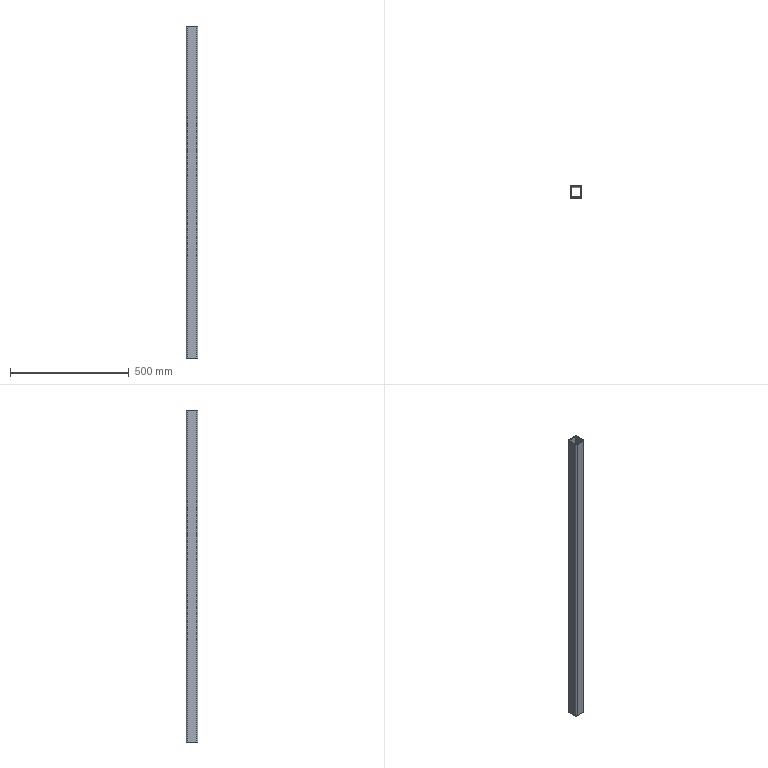Part | SolidWorks | features Extrusion 1 | 1 solid | 18 faces | box 50 x 50 x 1400 mm | volume 1217938 mm3 | plane 10 | cylinder 8 | commonest cylinder face diameters 2 x4 12 x4
STEP:
#1=CARTESIAN_POINT('',(0.,6.,1400.));
#2=VERTEX_POINT('',#1);
#3=CARTESIAN_POINT('',(6.,0.,1400.));
#4=VERTEX_POINT('',#3);
#5=CARTESIAN_POINT('',(6.,6.,1400.));
#6=DIRECTION('',(0.,0.,1.));
#7=DIRECTION('',(-1.,0.,0.));
#8=AXIS2_PLACEMENT_3D('',#5,#6,#7);
#9=CIRCLE('',#8,6.);
#10=EDGE_CURVE('',#2,#4,#9,.T.);
#11=ORIENTED_EDGE('',*,*,#10,.T.);
#12=CARTESIAN_POINT('',(44.,0.,1400.));
#13=VERTEX_POINT('',#12);
#14=CARTESIAN_POINT('',(6.,0.,1400.));
#15=DIRECTION('',(1.,0.,0.));
#16=VECTOR('',#15,1000.);
#17=LINE('',#14,#16);
#18=EDGE_CURVE('',#4,#13,#17,.T.);
#19=ORIENTED_EDGE('',*,*,#18,.T.);
#20=CARTESIAN_POINT('',(50.,6.,1400.));
#21=VERTEX_POINT('',#20);
#22=CARTESIAN_POINT('',(44.,6.,1400.));
#23=DIRECTION('',(0.,0.,1.));
#24=DIRECTION('',(1.,0.,0.));
#25=AXIS2_PLACEMENT_3D('',#22,#23,#24);
#26=CIRCLE('',#25,6.);
#27=EDGE_CURVE('',#13,#21,#26,.T.);
#28=ORIENTED_EDGE('',*,*,#27,.T.);
#29=CARTESIAN_POINT('',(50.,44.,1400.));
#30=VERTEX_POINT('',#29);
#31=CARTESIAN_POINT('',(50.,6.,1400.));
#32=DIRECTION('',(0.,1.,0.));
#33=VECTOR('',#32,1000.);
#34=LINE('',#31,#33);
#35=EDGE_CURVE('',#21,#30,#34,.T.);
#36=ORIENTED_EDGE('',*,*,#35,.T.);
#37=CARTESIAN_POINT('',(44.,50.,1400.));
#38=VERTEX_POINT('',#37);
#39=CARTESIAN_POINT('',(44.,44.,1400.));
#40=DIRECTION('',(0.,0.,1.));
#41=DIRECTION('',(-1.,0.,0.));
#42=AXIS2_PLACEMENT_3D('',#39,#40,#41);
#43=CIRCLE('',#42,6.);
#44=EDGE_CURVE('',#30,#38,#43,.T.);
#45=ORIENTED_EDGE('',*,*,#44,.T.);
#46=CARTESIAN_POINT('',(6.,50.,1400.));
#47=VERTEX_POINT('',#46);
#48=CARTESIAN_POINT('',(6.,50.,1400.));
#49=DIRECTION('',(-1.,0.,0.));
#50=VECTOR('',#49,1000.);
#51=LINE('',#48,#50);
#52=EDGE_CURVE('',#38,#47,#51,.T.);
#53=ORIENTED_EDGE('',*,*,#52,.T.);
#54=CARTESIAN_POINT('',(0.,44.,1400.));
#55=VERTEX_POINT('',#54);
#56=CARTESIAN_POINT('',(6.,44.,1400.));
#57=DIRECTION('',(0.,0.,1.));
#58=DIRECTION('',(-1.,0.,0.));
#59=AXIS2_PLACEMENT_3D('',#56,#57,#58);
#60=CIRCLE('',#59,6.);
#61=EDGE_CURVE('',#47,#55,#60,.T.);
#62=ORIENTED_EDGE('',*,*,#61,.T.);
#63=CARTESIAN_POINT('',(0.,6.,1400.));
#64=DIRECTION('',(0.,-1.,0.));
#65=VECTOR('',#64,1000.);
#66=LINE('',#63,#65);
#67=EDGE_CURVE('',#55,#2,#66,.T.);
#68=ORIENTED_EDGE('',*,*,#67,.T.);
#69=EDGE_LOOP('',(#11,#19,#28,#36,#45,#53,#62,#68));
#70=FACE_OUTER_BOUND('',#69,.T.);
#71=CARTESIAN_POINT('',(6.,45.,1400.));
#72=VERTEX_POINT('',#71);
#73=CARTESIAN_POINT('',(5.,44.,1400.));
#74=VERTEX_POINT('',#73);
#75=CARTESIAN_POINT('',(6.,44.,1400.));
#76=DIRECTION('',(0.,0.,1.));
#77=DIRECTION('',(-1.,0.,0.));
#78=AXIS2_PLACEMENT_3D('',#75,#76,#77);
#79=CIRCLE('',#78,1.);
#80=EDGE_CURVE('',#72,#74,#79,.T.);
#81=ORIENTED_EDGE('',*,*,#80,.F.);
#82=CARTESIAN_POINT('',(44.,45.,1400.));
#83=VERTEX_POINT('',#82);
#84=CARTESIAN_POINT('',(6.,45.,1400.));
#85=DIRECTION('',(-1.,0.,0.));
#86=VECTOR('',#85,1000.);
#87=LINE('',#84,#86);
#88=EDGE_CURVE('',#83,#72,#87,.T.);
#89=ORIENTED_EDGE('',*,*,#88,.F.);
#90=CARTESIAN_POINT('',(45.,44.,1400.));
#91=VERTEX_POINT('',#90);
#92=CARTESIAN_POINT('',(44.,44.,1400.));
#93=DIRECTION('',(0.,0.,1.));
#94=DIRECTION('',(-1.,0.,0.));
#95=AXIS2_PLACEMENT_3D('',#92,#93,#94);
#96=CIRCLE('',#95,1.);
#97=EDGE_CURVE('',#91,#83,#96,.T.);
#98=ORIENTED_EDGE('',*,*,#97,.F.);
#99=CARTESIAN_POINT('',(45.,6.,1400.));
#100=VERTEX_POINT('',#99);
#101=CARTESIAN_POINT('',(45.,6.,1400.));
#102=DIRECTION('',(0.,1.,0.));
#103=VECTOR('',#102,1000.);
#104=LINE('',#101,#103);
#105=EDGE_CURVE('',#100,#91,#104,.T.);
#106=ORIENTED_EDGE('',*,*,#105,.F.);
#107=CARTESIAN_POINT('',(44.,5.,1400.));
#108=VERTEX_POINT('',#107);
#109=CARTESIAN_POINT('',(44.,6.,1400.));
#110=DIRECTION('',(0.,0.,1.));
#111=DIRECTION('',(1.,0.,0.));
#112=AXIS2_PLACEMENT_3D('',#109,#110,#111);
#113=CIRCLE('',#112,1.);
#114=EDGE_CURVE('',#108,#100,#113,.T.);
#115=ORIENTED_EDGE('',*,*,#114,.F.);
#116=CARTESIAN_POINT('',(6.,5.,1400.));
#117=VERTEX_POINT('',#116);
#118=CARTESIAN_POINT('',(6.,5.,1400.));
#119=DIRECTION('',(1.,0.,0.));
#120=VECTOR('',#119,1000.);
#121=LINE('',#118,#120);
#122=EDGE_CURVE('',#117,#108,#121,.T.);
#123=ORIENTED_EDGE('',*,*,#122,.F.);
#124=CARTESIAN_POINT('',(5.,6.,1400.));
#125=VERTEX_POINT('',#124);
#126=CARTESIAN_POINT('',(6.,6.,1400.));
#127=DIRECTION('',(0.,0.,1.));
#128=DIRECTION('',(-1.,0.,0.));
#129=AXIS2_PLACEMENT_3D('',#126,#127,#128);
#130=CIRCLE('',#129,1.);
#131=EDGE_CURVE('',#125,#117,#130,.T.);
#132=ORIENTED_EDGE('',*,*,#131,.F.);
#133=CARTESIAN_POINT('',(5.,6.,1400.));
#134=DIRECTION('',(0.,-1.,0.));
#135=VECTOR('',#134,1000.);
#136=LINE('',#133,#135);
#137=EDGE_CURVE('',#74,#125,#136,.T.);
#138=ORIENTED_EDGE('',*,*,#137,.F.);
#139=EDGE_LOOP('',(#81,#89,#98,#106,#115,#123,#132,#138));
#140=FACE_BOUND('',#139,.T.);
#141=CARTESIAN_POINT('',(6.,6.,1400.));
#142=DIRECTION('',(0.,0.,-1.));
#143=DIRECTION('',(-1.,0.,0.));
#144=AXIS2_PLACEMENT_3D('',#141,#142,#143);
#145=PLANE('',#144);
#146=ADVANCED_FACE('',(#70,#140),#145,.F.);
#147=CARTESIAN_POINT('',(0.,6.,0.));
#148=VERTEX_POINT('',#147);
#149=CARTESIAN_POINT('',(6.,0.,0.));
#150=VERTEX_POINT('',#149);
#151=CARTESIAN_POINT('',(6.,6.,0.));
#152=DIRECTION('',(0.,0.,1.));
#153=DIRECTION('',(-1.,0.,0.));
#154=AXIS2_PLACEMENT_3D('',#151,#152,#153);
#155=CIRCLE('',#154,6.);
#156=EDGE_CURVE('',#148,#150,#155,.T.);
#157=ORIENTED_EDGE('',*,*,#156,.F.);
#158=CARTESIAN_POINT('',(0.,44.,0.));
#159=VERTEX_POINT('',#158);
#160=CARTESIAN_POINT('',(0.,6.,0.));
#161=DIRECTION('',(0.,-1.,0.));
#162=VECTOR('',#161,1000.);
#163=LINE('',#160,#162);
#164=EDGE_CURVE('',#159,#148,#163,.T.);
#165=ORIENTED_EDGE('',*,*,#164,.F.);
#166=CARTESIAN_POINT('',(6.,50.,0.));
#167=VERTEX_POINT('',#166);
#168=CARTESIAN_POINT('',(6.,44.,0.));
#169=DIRECTION('',(0.,0.,1.));
#170=DIRECTION('',(-1.,0.,0.));
#171=AXIS2_PLACEMENT_3D('',#168,#169,#170);
#172=CIRCLE('',#171,6.);
#173=EDGE_CURVE('',#167,#159,#172,.T.);
#174=ORIENTED_EDGE('',*,*,#173,.F.);
#175=CARTESIAN_POINT('',(44.,50.,0.));
#176=VERTEX_POINT('',#175);
#177=CARTESIAN_POINT('',(6.,50.,0.));
#178=DIRECTION('',(-1.,0.,0.));
#179=VECTOR('',#178,1000.);
#180=LINE('',#177,#179);
#181=EDGE_CURVE('',#176,#167,#180,.T.);
#182=ORIENTED_EDGE('',*,*,#181,.F.);
#183=CARTESIAN_POINT('',(50.,44.,0.));
#184=VERTEX_POINT('',#183);
#185=CARTESIAN_POINT('',(44.,44.,0.));
#186=DIRECTION('',(0.,0.,1.));
#187=DIRECTION('',(-1.,0.,0.));
#188=AXIS2_PLACEMENT_3D('',#185,#186,#187);
#189=CIRCLE('',#188,6.);
#190=EDGE_CURVE('',#184,#176,#189,.T.);
#191=ORIENTED_EDGE('',*,*,#190,.F.);
#192=CARTESIAN_POINT('',(50.,6.,0.));
#193=VERTEX_POINT('',#192);
#194=CARTESIAN_POINT('',(50.,6.,0.));
#195=DIRECTION('',(0.,1.,0.));
#196=VECTOR('',#195,1000.);
#197=LINE('',#194,#196);
#198=EDGE_CURVE('',#193,#184,#197,.T.);
#199=ORIENTED_EDGE('',*,*,#198,.F.);
#200=CARTESIAN_POINT('',(44.,0.,0.));
#201=VERTEX_POINT('',#200);
#202=CARTESIAN_POINT('',(44.,6.,0.));
#203=DIRECTION('',(0.,0.,1.));
#204=DIRECTION('',(1.,0.,0.));
#205=AXIS2_PLACEMENT_3D('',#202,#203,#204);
#206=CIRCLE('',#205,6.);
#207=EDGE_CURVE('',#201,#193,#206,.T.);
#208=ORIENTED_EDGE('',*,*,#207,.F.);
#209=CARTESIAN_POINT('',(6.,0.,0.));
#210=DIRECTION('',(1.,0.,0.));
#211=VECTOR('',#210,1000.);
#212=LINE('',#209,#211);
#213=EDGE_CURVE('',#150,#201,#212,.T.);
#214=ORIENTED_EDGE('',*,*,#213,.F.);
#215=EDGE_LOOP('',(#157,#165,#174,#182,#191,#199,#208,#214));
#216=FACE_OUTER_BOUND('',#215,.T.);
#217=CARTESIAN_POINT('',(44.,45.,0.));
#218=VERTEX_POINT('',#217);
#219=CARTESIAN_POINT('',(6.,45.,0.));
#220=VERTEX_POINT('',#219);
#221=CARTESIAN_POINT('',(6.,45.,0.));
#222=DIRECTION('',(-1.,0.,0.));
#223=VECTOR('',#222,1000.);
#224=LINE('',#221,#223);
#225=EDGE_CURVE('',#218,#220,#224,.T.);
#226=ORIENTED_EDGE('',*,*,#225,.T.);
#227=CARTESIAN_POINT('',(5.,44.,0.));
#228=VERTEX_POINT('',#227);
#229=CARTESIAN_POINT('',(6.,44.,0.));
#230=DIRECTION('',(0.,0.,1.));
#231=DIRECTION('',(-1.,0.,0.));
#232=AXIS2_PLACEMENT_3D('',#229,#230,#231);
#233=CIRCLE('',#232,1.);
#234=EDGE_CURVE('',#220,#228,#233,.T.);
#235=ORIENTED_EDGE('',*,*,#234,.T.);
#236=CARTESIAN_POINT('',(5.,6.,0.));
#237=VERTEX_POINT('',#236);
#238=CARTESIAN_POINT('',(5.,6.,0.));
#239=DIRECTION('',(0.,-1.,0.));
#240=VECTOR('',#239,1000.);
#241=LINE('',#238,#240);
#242=EDGE_CURVE('',#228,#237,#241,.T.);
#243=ORIENTED_EDGE('',*,*,#242,.T.);
#244=CARTESIAN_POINT('',(6.,5.,0.));
#245=VERTEX_POINT('',#244);
#246=CARTESIAN_POINT('',(6.,6.,0.));
#247=DIRECTION('',(0.,0.,1.));
#248=DIRECTION('',(-1.,0.,0.));
#249=AXIS2_PLACEMENT_3D('',#246,#247,#248);
#250=CIRCLE('',#249,1.);
#251=EDGE_CURVE('',#237,#245,#250,.T.);
#252=ORIENTED_EDGE('',*,*,#251,.T.);
#253=CARTESIAN_POINT('',(44.,5.,0.));
#254=VERTEX_POINT('',#253);
#255=CARTESIAN_POINT('',(6.,5.,0.));
#256=DIRECTION('',(1.,0.,0.));
#257=VECTOR('',#256,1000.);
#258=LINE('',#255,#257);
#259=EDGE_CURVE('',#245,#254,#258,.T.);
#260=ORIENTED_EDGE('',*,*,#259,.T.);
#261=CARTESIAN_POINT('',(45.,6.,0.));
#262=VERTEX_POINT('',#261);
#263=CARTESIAN_POINT('',(44.,6.,0.));
#264=DIRECTION('',(0.,0.,1.));
#265=DIRECTION('',(1.,0.,0.));
#266=AXIS2_PLACEMENT_3D('',#263,#264,#265);
#267=CIRCLE('',#266,1.);
#268=EDGE_CURVE('',#254,#262,#267,.T.);
#269=ORIENTED_EDGE('',*,*,#268,.T.);
#270=CARTESIAN_POINT('',(45.,44.,0.));
#271=VERTEX_POINT('',#270);
#272=CARTESIAN_POINT('',(45.,6.,0.));
#273=DIRECTION('',(0.,1.,0.));
#274=VECTOR('',#273,1000.);
#275=LINE('',#272,#274);
#276=EDGE_CURVE('',#262,#271,#275,.T.);
#277=ORIENTED_EDGE('',*,*,#276,.T.);
#278=CARTESIAN_POINT('',(44.,44.,0.));
#279=DIRECTION('',(0.,0.,1.));
#280=DIRECTION('',(-1.,0.,0.));
#281=AXIS2_PLACEMENT_3D('',#278,#279,#280);
#282=CIRCLE('',#281,1.);
#283=EDGE_CURVE('',#271,#218,#282,.T.);
#284=ORIENTED_EDGE('',*,*,#283,.T.);
#285=EDGE_LOOP('',(#226,#235,#243,#252,#260,#269,#277,#284));
#286=FACE_BOUND('',#285,.T.);
#287=CARTESIAN_POINT('',(6.,6.,0.));
#288=DIRECTION('',(0.,0.,-1.));
#289=DIRECTION('',(-1.,0.,0.));
#290=AXIS2_PLACEMENT_3D('',#287,#288,#289);
#291=PLANE('',#290);
#292=ADVANCED_FACE('',(#216,#286),#291,.T.);
#293=ORIENTED_EDGE('',*,*,#156,.T.);
#294=CARTESIAN_POINT('',(6.,0.,1400.));
#295=DIRECTION('',(0.,0.,-1.));
#296=VECTOR('',#295,1000.);
#297=LINE('',#294,#296);
#298=EDGE_CURVE('',#4,#150,#297,.T.);
#299=ORIENTED_EDGE('',*,*,#298,.F.);
#300=ORIENTED_EDGE('',*,*,#10,.F.);
#301=CARTESIAN_POINT('',(0.,6.,1400.));
#302=DIRECTION('',(0.,0.,-1.));
#303=VECTOR('',#302,1000.);
#304=LINE('',#301,#303);
#305=EDGE_CURVE('',#2,#148,#304,.T.);
#306=ORIENTED_EDGE('',*,*,#305,.T.);
#307=EDGE_LOOP('',(#293,#299,#300,#306));
#308=FACE_OUTER_BOUND('',#307,.T.);
#309=CARTESIAN_POINT('',(6.,6.,1400.));
#310=DIRECTION('',(0.,0.,-1.));
#311=DIRECTION('',(-1.,0.,0.));
#312=AXIS2_PLACEMENT_3D('',#309,#310,#311);
#313=CYLINDRICAL_SURFACE('',#312,6.);
#314=ADVANCED_FACE('',(#308),#313,.T.);
#315=ORIENTED_EDGE('',*,*,#213,.T.);
#316=CARTESIAN_POINT('',(44.,0.,1400.));
#317=DIRECTION('',(0.,0.,-1.));
#318=VECTOR('',#317,1000.);
#319=LINE('',#316,#318);
#320=EDGE_CURVE('',#13,#201,#319,.T.);
#321=ORIENTED_EDGE('',*,*,#320,.F.);
#322=ORIENTED_EDGE('',*,*,#18,.F.);
#323=ORIENTED_EDGE('',*,*,#298,.T.);
#324=EDGE_LOOP('',(#315,#321,#322,#323));
#325=FACE_OUTER_BOUND('',#324,.T.);
#326=CARTESIAN_POINT('',(6.,0.,1400.));
#327=DIRECTION('',(0.,1.,0.));
#328=DIRECTION('',(0.,0.,1.));
#329=AXIS2_PLACEMENT_3D('',#326,#327,#328);
#330=PLANE('',#329);
#331=ADVANCED_FACE('',(#325),#330,.F.);
#332=ORIENTED_EDGE('',*,*,#207,.T.);
#333=CARTESIAN_POINT('',(50.,6.,1400.));
#334=DIRECTION('',(0.,0.,-1.));
#335=VECTOR('',#334,1000.);
#336=LINE('',#333,#335);
#337=EDGE_CURVE('',#21,#193,#336,.T.);
#338=ORIENTED_EDGE('',*,*,#337,.F.);
#339=ORIENTED_EDGE('',*,*,#27,.F.);
#340=ORIENTED_EDGE('',*,*,#320,.T.);
#341=EDGE_LOOP('',(#332,#338,#339,#340));
#342=FACE_OUTER_BOUND('',#341,.T.);
#343=CARTESIAN_POINT('',(44.,6.,1400.));
#344=DIRECTION('',(0.,0.,-1.));
#345=DIRECTION('',(-1.,0.,0.));
#346=AXIS2_PLACEMENT_3D('',#343,#344,#345);
#347=CYLINDRICAL_SURFACE('',#346,6.);
#348=ADVANCED_FACE('',(#342),#347,.T.);
#349=ORIENTED_EDGE('',*,*,#198,.T.);
#350=CARTESIAN_POINT('',(50.,44.,1400.));
#351=DIRECTION('',(0.,0.,-1.));
#352=VECTOR('',#351,1000.);
#353=LINE('',#350,#352);
#354=EDGE_CURVE('',#30,#184,#353,.T.);
#355=ORIENTED_EDGE('',*,*,#354,.F.);
#356=ORIENTED_EDGE('',*,*,#35,.F.);
#357=ORIENTED_EDGE('',*,*,#337,.T.);
#358=EDGE_LOOP('',(#349,#355,#356,#357));
#359=FACE_OUTER_BOUND('',#358,.T.);
#360=CARTESIAN_POINT('',(50.,6.,1400.));
#361=DIRECTION('',(-1.,0.,0.));
#362=DIRECTION('',(0.,0.,1.));
#363=AXIS2_PLACEMENT_3D('',#360,#361,#362);
#364=PLANE('',#363);
#365=ADVANCED_FACE('',(#359),#364,.F.);
#366=ORIENTED_EDGE('',*,*,#190,.T.);
#367=CARTESIAN_POINT('',(44.,50.,1400.));
#368=DIRECTION('',(0.,0.,-1.));
#369=VECTOR('',#368,1000.);
#370=LINE('',#367,#369);
#371=EDGE_CURVE('',#38,#176,#370,.T.);
#372=ORIENTED_EDGE('',*,*,#371,.F.);
#373=ORIENTED_EDGE('',*,*,#44,.F.);
#374=ORIENTED_EDGE('',*,*,#354,.T.);
#375=EDGE_LOOP('',(#366,#372,#373,#374));
#376=FACE_OUTER_BOUND('',#375,.T.);
#377=CARTESIAN_POINT('',(44.,44.,1400.));
#378=DIRECTION('',(0.,0.,-1.));
#379=DIRECTION('',(-1.,0.,0.));
#380=AXIS2_PLACEMENT_3D('',#377,#378,#379);
#381=CYLINDRICAL_SURFACE('',#380,6.);
#382=ADVANCED_FACE('',(#376),#381,.T.);
#383=ORIENTED_EDGE('',*,*,#181,.T.);
#384=CARTESIAN_POINT('',(6.,50.,1400.));
#385=DIRECTION('',(0.,0.,-1.));
#386=VECTOR('',#385,1000.);
#387=LINE('',#384,#386);
#388=EDGE_CURVE('',#47,#167,#387,.T.);
#389=ORIENTED_EDGE('',*,*,#388,.F.);
#390=ORIENTED_EDGE('',*,*,#52,.F.);
#391=ORIENTED_EDGE('',*,*,#371,.T.);
#392=EDGE_LOOP('',(#383,#389,#390,#391));
#393=FACE_OUTER_BOUND('',#392,.T.);
#394=CARTESIAN_POINT('',(6.,50.,1400.));
#395=DIRECTION('',(0.,-1.,0.));
#396=DIRECTION('',(0.,0.,-1.));
#397=AXIS2_PLACEMENT_3D('',#394,#395,#396);
#398=PLANE('',#397);
#399=ADVANCED_FACE('',(#393),#398,.F.);
#400=ORIENTED_EDGE('',*,*,#173,.T.);
#401=CARTESIAN_POINT('',(0.,44.,1400.));
#402=DIRECTION('',(0.,0.,-1.));
#403=VECTOR('',#402,1000.);
#404=LINE('',#401,#403);
#405=EDGE_CURVE('',#55,#159,#404,.T.);
#406=ORIENTED_EDGE('',*,*,#405,.F.);
#407=ORIENTED_EDGE('',*,*,#61,.F.);
#408=ORIENTED_EDGE('',*,*,#388,.T.);
#409=EDGE_LOOP('',(#400,#406,#407,#408));
#410=FACE_OUTER_BOUND('',#409,.T.);
#411=CARTESIAN_POINT('',(6.,44.,1400.));
#412=DIRECTION('',(0.,0.,-1.));
#413=DIRECTION('',(-1.,0.,0.));
#414=AXIS2_PLACEMENT_3D('',#411,#412,#413);
#415=CYLINDRICAL_SURFACE('',#414,6.);
#416=ADVANCED_FACE('',(#410),#415,.T.);
#417=ORIENTED_EDGE('',*,*,#164,.T.);
#418=ORIENTED_EDGE('',*,*,#305,.F.);
#419=ORIENTED_EDGE('',*,*,#67,.F.);
#420=ORIENTED_EDGE('',*,*,#405,.T.);
#421=EDGE_LOOP('',(#417,#418,#419,#420));
#422=FACE_OUTER_BOUND('',#421,.T.);
#423=CARTESIAN_POINT('',(0.,6.,1400.));
#424=DIRECTION('',(1.,0.,0.));
#425=DIRECTION('',(0.,0.,-1.));
#426=AXIS2_PLACEMENT_3D('',#423,#424,#425);
#427=PLANE('',#426);
#428=ADVANCED_FACE('',(#422),#427,.F.);
#429=ORIENTED_EDGE('',*,*,#234,.F.);
#430=CARTESIAN_POINT('',(6.,45.,1400.));
#431=DIRECTION('',(0.,0.,-1.));
#432=VECTOR('',#431,1000.);
#433=LINE('',#430,#432);
#434=EDGE_CURVE('',#72,#220,#433,.T.);
#435=ORIENTED_EDGE('',*,*,#434,.F.);
#436=ORIENTED_EDGE('',*,*,#80,.T.);
#437=CARTESIAN_POINT('',(5.,44.,1400.));
#438=DIRECTION('',(0.,0.,-1.));
#439=VECTOR('',#438,1000.);
#440=LINE('',#437,#439);
#441=EDGE_CURVE('',#74,#228,#440,.T.);
#442=ORIENTED_EDGE('',*,*,#441,.T.);
#443=EDGE_LOOP('',(#429,#435,#436,#442));
#444=FACE_OUTER_BOUND('',#443,.T.);
#445=CARTESIAN_POINT('',(6.,44.,1400.));
#446=DIRECTION('',(0.,0.,-1.));
#447=DIRECTION('',(-1.,0.,0.));
#448=AXIS2_PLACEMENT_3D('',#445,#446,#447);
#449=CYLINDRICAL_SURFACE('',#448,1.);
#450=ADVANCED_FACE('',(#444),#449,.F.);
#451=ORIENTED_EDGE('',*,*,#242,.F.);
#452=ORIENTED_EDGE('',*,*,#441,.F.);
#453=ORIENTED_EDGE('',*,*,#137,.T.);
#454=CARTESIAN_POINT('',(5.,6.,1400.));
#455=DIRECTION('',(0.,0.,-1.));
#456=VECTOR('',#455,1000.);
#457=LINE('',#454,#456);
#458=EDGE_CURVE('',#125,#237,#457,.T.);
#459=ORIENTED_EDGE('',*,*,#458,.T.);
#460=EDGE_LOOP('',(#451,#452,#453,#459));
#461=FACE_OUTER_BOUND('',#460,.T.);
#462=CARTESIAN_POINT('',(5.,6.,1400.));
#463=DIRECTION('',(1.,0.,0.));
#464=DIRECTION('',(0.,1.,0.));
#465=AXIS2_PLACEMENT_3D('',#462,#463,#464);
#466=PLANE('',#465);
#467=ADVANCED_FACE('',(#461),#466,.T.);
#468=ORIENTED_EDGE('',*,*,#251,.F.);
#469=ORIENTED_EDGE('',*,*,#458,.F.);
#470=ORIENTED_EDGE('',*,*,#131,.T.);
#471=CARTESIAN_POINT('',(6.,5.,1400.));
#472=DIRECTION('',(0.,0.,-1.));
#473=VECTOR('',#472,1000.);
#474=LINE('',#471,#473);
#475=EDGE_CURVE('',#117,#245,#474,.T.);
#476=ORIENTED_EDGE('',*,*,#475,.T.);
#477=EDGE_LOOP('',(#468,#469,#470,#476));
#478=FACE_OUTER_BOUND('',#477,.T.);
#479=CARTESIAN_POINT('',(6.,6.,1400.));
#480=DIRECTION('',(0.,0.,-1.));
#481=DIRECTION('',(-1.,0.,0.));
#482=AXIS2_PLACEMENT_3D('',#479,#480,#481);
#483=CYLINDRICAL_SURFACE('',#482,1.);
#484=ADVANCED_FACE('',(#478),#483,.F.);
#485=ORIENTED_EDGE('',*,*,#259,.F.);
#486=ORIENTED_EDGE('',*,*,#475,.F.);
#487=ORIENTED_EDGE('',*,*,#122,.T.);
#488=CARTESIAN_POINT('',(44.,5.,1400.));
#489=DIRECTION('',(0.,0.,-1.));
#490=VECTOR('',#489,1000.);
#491=LINE('',#488,#490);
#492=EDGE_CURVE('',#108,#254,#491,.T.);
#493=ORIENTED_EDGE('',*,*,#492,.T.);
#494=EDGE_LOOP('',(#485,#486,#487,#493));
#495=FACE_OUTER_BOUND('',#494,.T.);
#496=CARTESIAN_POINT('',(6.,5.,1400.));
#497=DIRECTION('',(0.,1.,0.));
#498=DIRECTION('',(-1.,0.,0.));
#499=AXIS2_PLACEMENT_3D('',#496,#497,#498);
#500=PLANE('',#499);
#501=ADVANCED_FACE('',(#495),#500,.T.);
#502=ORIENTED_EDGE('',*,*,#268,.F.);
#503=ORIENTED_EDGE('',*,*,#492,.F.);
#504=ORIENTED_EDGE('',*,*,#114,.T.);
#505=CARTESIAN_POINT('',(45.,6.,1400.));
#506=DIRECTION('',(0.,0.,-1.));
#507=VECTOR('',#506,1000.);
#508=LINE('',#505,#507);
#509=EDGE_CURVE('',#100,#262,#508,.T.);
#510=ORIENTED_EDGE('',*,*,#509,.T.);
#511=EDGE_LOOP('',(#502,#503,#504,#510));
#512=FACE_OUTER_BOUND('',#511,.T.);
#513=CARTESIAN_POINT('',(44.,6.,1400.));
#514=DIRECTION('',(0.,0.,-1.));
#515=DIRECTION('',(-1.,0.,0.));
#516=AXIS2_PLACEMENT_3D('',#513,#514,#515);
#517=CYLINDRICAL_SURFACE('',#516,1.);
#518=ADVANCED_FACE('',(#512),#517,.F.);
#519=ORIENTED_EDGE('',*,*,#276,.F.);
#520=ORIENTED_EDGE('',*,*,#509,.F.);
#521=ORIENTED_EDGE('',*,*,#105,.T.);
#522=CARTESIAN_POINT('',(45.,44.,1400.));
#523=DIRECTION('',(0.,0.,-1.));
#524=VECTOR('',#523,1000.);
#525=LINE('',#522,#524);
#526=EDGE_CURVE('',#91,#271,#525,.T.);
#527=ORIENTED_EDGE('',*,*,#526,.T.);
#528=EDGE_LOOP('',(#519,#520,#521,#527));
#529=FACE_OUTER_BOUND('',#528,.T.);
#530=CARTESIAN_POINT('',(45.,6.,1400.));
#531=DIRECTION('',(-1.,0.,0.));
#532=DIRECTION('',(0.,0.,1.));
#533=AXIS2_PLACEMENT_3D('',#530,#531,#532);
#534=PLANE('',#533);
#535=ADVANCED_FACE('',(#529),#534,.T.);
#536=ORIENTED_EDGE('',*,*,#283,.F.);
#537=ORIENTED_EDGE('',*,*,#526,.F.);
#538=ORIENTED_EDGE('',*,*,#97,.T.);
#539=CARTESIAN_POINT('',(44.,45.,1400.));
#540=DIRECTION('',(0.,0.,-1.));
#541=VECTOR('',#540,1000.);
#542=LINE('',#539,#541);
#543=EDGE_CURVE('',#83,#218,#542,.T.);
#544=ORIENTED_EDGE('',*,*,#543,.T.);
#545=EDGE_LOOP('',(#536,#537,#538,#544));
#546=FACE_OUTER_BOUND('',#545,.T.);
#547=CARTESIAN_POINT('',(44.,44.,1400.));
#548=DIRECTION('',(0.,0.,-1.));
#549=DIRECTION('',(-1.,0.,0.));
#550=AXIS2_PLACEMENT_3D('',#547,#548,#549);
#551=CYLINDRICAL_SURFACE('',#550,1.);
#552=ADVANCED_FACE('',(#546),#551,.F.);
#553=ORIENTED_EDGE('',*,*,#225,.F.);
#554=ORIENTED_EDGE('',*,*,#543,.F.);
#555=ORIENTED_EDGE('',*,*,#88,.T.);
#556=ORIENTED_EDGE('',*,*,#434,.T.);
#557=EDGE_LOOP('',(#553,#554,#555,#556));
#558=FACE_OUTER_BOUND('',#557,.T.);
#559=CARTESIAN_POINT('',(6.,45.,1400.));
#560=DIRECTION('',(0.,-1.,0.));
#561=DIRECTION('',(0.,0.,-1.));
#562=AXIS2_PLACEMENT_3D('',#559,#560,#561);
#563=PLANE('',#562);
#564=ADVANCED_FACE('',(#558),#563,.T.);
#565=CLOSED_SHELL('',(#146,#292,#314,#331,#348,#365,#382,#399,#416,#428,#450,#467,#484,#501,#518,#535,#552,#564));
#566=MANIFOLD_SOLID_BREP('',#565);
#567=CARTESIAN_POINT('',(0.,0.,0.));
#568=DIRECTION('',(0.,0.,1.));
#569=DIRECTION('',(1.,0.,0.));
#570=AXIS2_PLACEMENT_3D('',#567,#568,#569);
#571=(LENGTH_UNIT()NAMED_UNIT(*)SI_UNIT(.MILLI.,.METRE.));
#572=UNCERTAINTY_MEASURE_WITH_UNIT(LENGTH_MEASURE(0.00001),#571,'','');
#573=(NAMED_UNIT(*)PLANE_ANGLE_UNIT()SI_UNIT($,.RADIAN.));
#574=(NAMED_UNIT(*)SI_UNIT($,.STERADIAN.)SOLID_ANGLE_UNIT());
#575=(GEOMETRIC_REPRESENTATION_CONTEXT(3)GLOBAL_UNCERTAINTY_ASSIGNED_CONTEXT((#572))GLOBAL_UNIT_ASSIGNED_CONTEXT((#571,#573,#574))REPRESENTATION_CONTEXT('',''));
#576=ADVANCED_BREP_SHAPE_REPRESENTATION('',(#566,#570),#575);